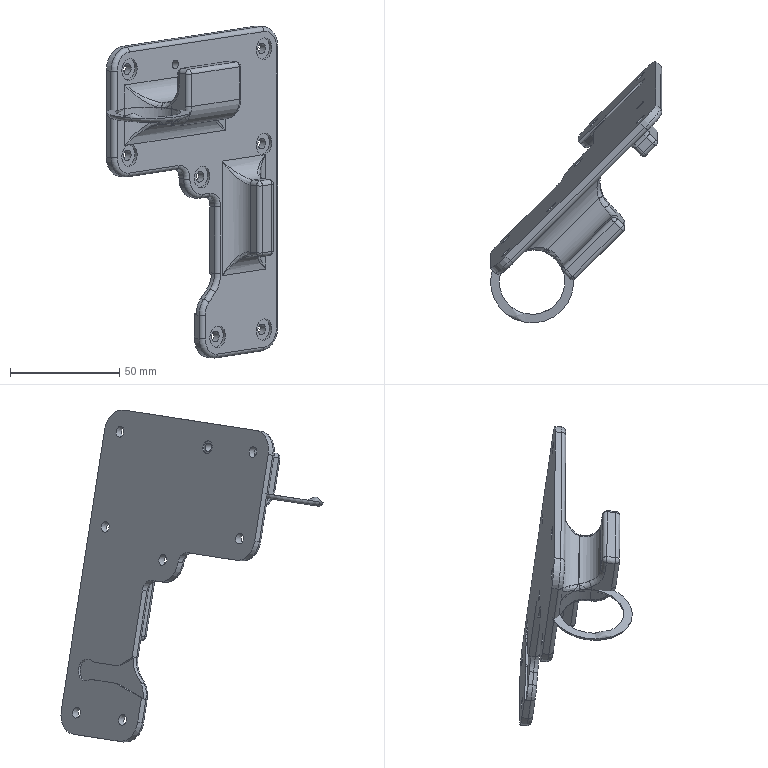Part | SolidWorks | features BaseBody 1 | 1 solid | 162 faces | box 78.368 x 119.921 x 151.933 mm | volume 75018 mm3 | cylinder 86 | plane 36 | torus 22 | spline 10 | sphere 8 | commonest cylinder face diameters 4 x29 10 x23 5 x14 20 x9 18 x7 6 x2